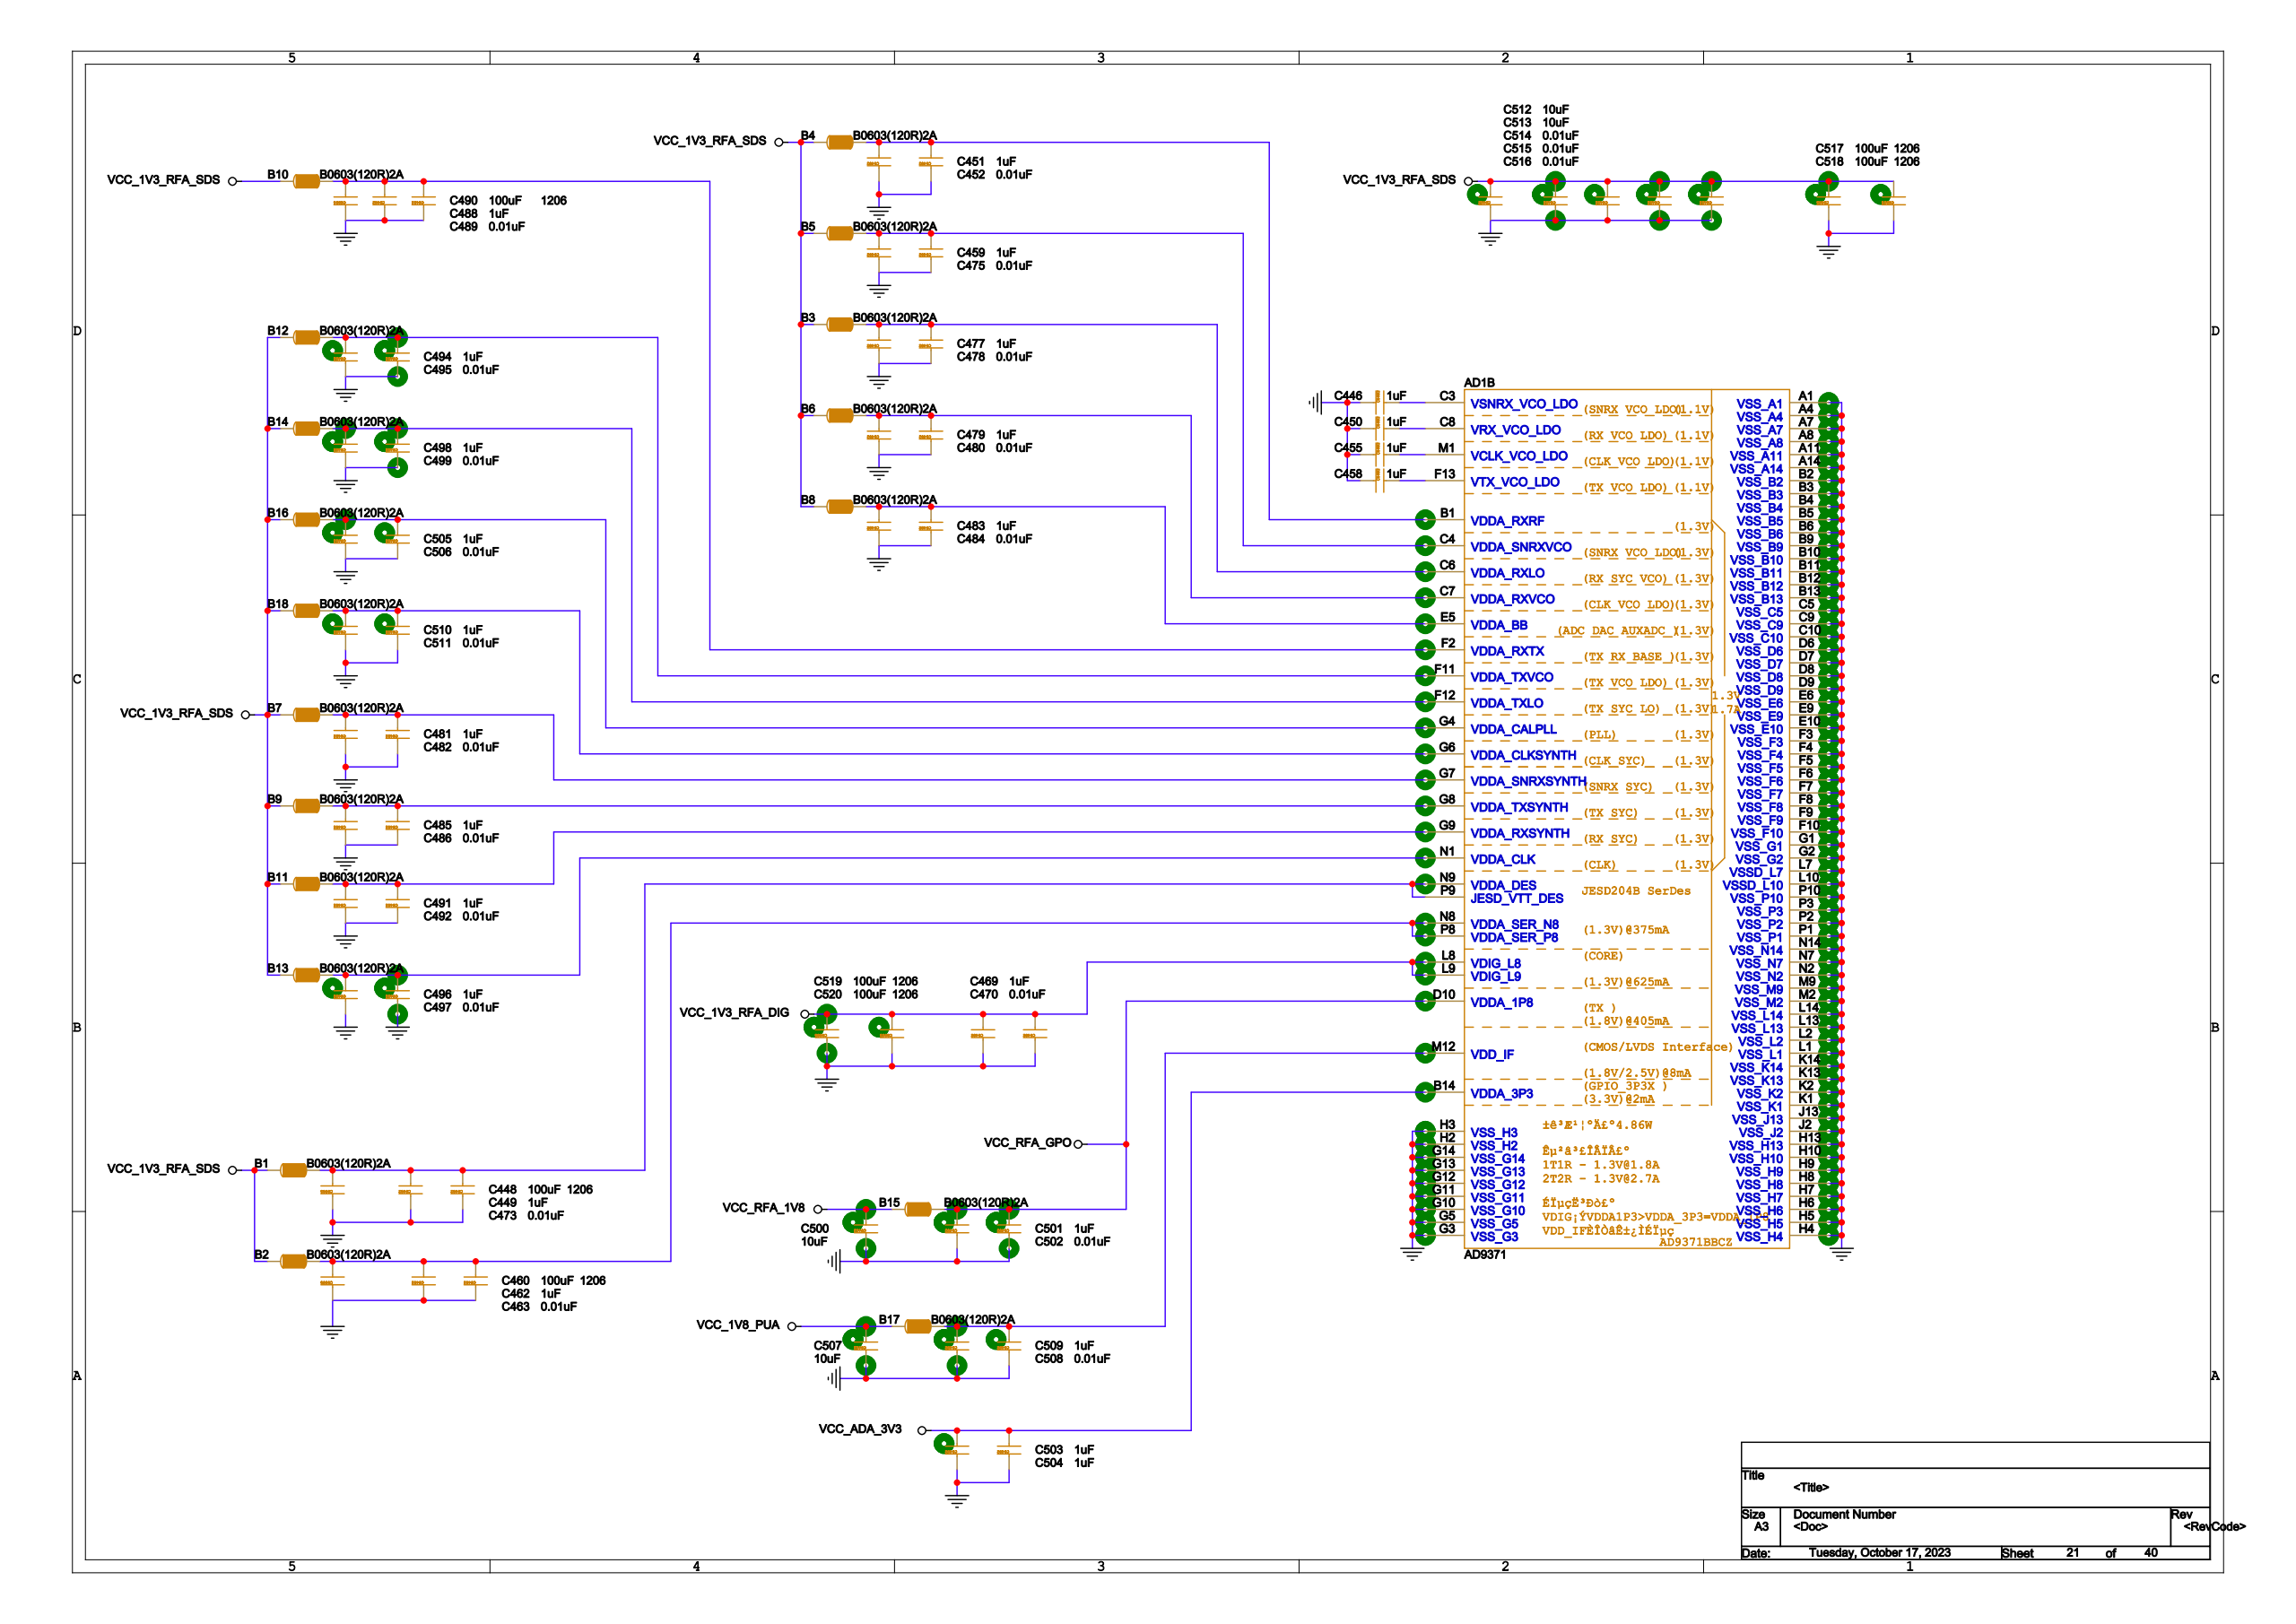Circuit board | Cadence Allegro | 1793 parts | 1223 nets | one sheet of the schematic
Parts on this sheet (reference | value | footprint):
AD1 | AD9371 | BGA196
B1 | B0603(120R)2A | B0603
B2 | B0603(120R)2A | B0603
B3 | B0603(120R)2A | B0603
B4 | B0603(120R)2A | B0603
B5 | B0603(120R)2A | B0603
B6 | B0603(120R)2A | B0603
B7 | B0603(120R)2A | B0603
B8 | B0603(120R)2A | B0603
B9 | B0603(120R)2A | B0603
B10 | B0603(120R)2A | B0603
B11 | B0603(120R)2A | B0603
B12 | B0603(120R)2A | B0603
B13 | B0603(120R)2A | B0603
B14 | B0603(120R)2A | B0603
B15 | B0603(120R)2A | B0603
B16 | B0603(120R)2A | B0603
B17 | B0603(120R)2A | B0603
B18 | B0603(120R)2A | B0603
C446 | 1uF | C0402
C448 | 100uF | 1206
C449 | 1uF | C0402
C450 | 1uF | C0402
C451 | 1uF | C0402
C452 | 0.01uF | C0402
C455 | 1uF | C0402
C458 | 1uF | C0402
C459 | 1uF | C0402
C460 | 100uF | 1206
C462 | 1uF | C0402
C463 | 0.01uF | C0402
C469 | 1uF | C0402
C470 | 0.01uF | C0402
C473 | 0.01uF | C0402
C475 | 0.01uF | C0402
C477 | 1uF | C0402
C478 | 0.01uF | C0402
C479 | 1uF | C0402
C480 | 0.01uF | C0402
C481 | 1uF | C0402
C482 | 0.01uF | C0402
C483 | 1uF | C0402
C484 | 0.01uF | C0402
C485 | 1uF | C0402
C486 | 0.01uF | C0402
C488 | 1uF | C0402
C489 | 0.01uF | C0402
C490 | 100uF | 1206
C491 | 1uF | C0402
C492 | 0.01uF | C0402
C494 | 1uF | C0402
C495 | 0.01uF | C0402
C496 | 1uF | C0402
C497 | 0.01uF | C0402
C498 | 1uF | C0402
C499 | 0.01uF | C0402
C500 | 10uF | C0402
C501 | 1uF | C0402
C502 | 0.01uF | C0402
C503 | 1uF | C0402
C504 | 1uF | C0402
C505 | 1uF | C0402
C506 | 0.01uF | C0402
C507 | 10uF | C0402
C508 | 0.01uF | C0402
C509 | 1uF | C0402
C510 | 1uF | C0402
C511 | 0.01uF | C0402
C512 | 10uF | C0402
C513 | 10uF | C0402
C514 | 0.01uF | C0402
C515 | 0.01uF | C0402
C516 | 0.01uF | C0402
C517 | 100uF | 1206
C518 | 100uF | 1206
C519 | 100uF | 1206
C520 | 100uF | 1206
Nets of these parts (net: part-pin ...):
GND: C446-1 C448-1 C449-1 C450-1 C451-1 C452-1 C455-1 C458-1 C459-1 C460-1 C462-1 C463-1 C469-1 C470-1 C473-1 C475-1 C477-1 C478-1 C479-1 C480-1 C481-1 C482-1 C483-1 C484-1 C485-1 C486-1 C488-1 C489-1 C490-1 C491-1 C492-1 C494-1 C495-1 C496-1 C497-1 C498-1 C499-1 C500-1 C501-1 C502-1 C503-1 C504-1 C505-1 C506-1 C507-1 C508-1 C509-1 C510-1 C511-1 C512-1 C513-1 C514-1 C515-1 C516-1 C517-1 C518-1 C519-1 C520-1 AD1-A1 AD1-A4 AD1-A7 AD1-A8 AD1-A11 AD1-A14 AD1-B2 AD1-B3 AD1-B4 AD1-B5 AD1-B6 AD1-B9 AD1-B10 AD1-B11 AD1-B12 AD1-B13 AD1-C5 AD1-C9 AD1-C10 AD1-D6 AD1-D7 AD1-D8 AD1-D9 AD1-E6 AD1-E9 AD1-E10 AD1-F3 AD1-F4 AD1-F5 AD1-F6 AD1-F7 AD1-F8 AD1-F9 AD1-F10 AD1-G1 AD1-G2 AD1-G3 AD1-G5 AD1-G10 AD1-G11 AD1-G12 AD1-G13 AD1-G14 AD1-H2 AD1-H3 AD1-H4 AD1-H5 AD1-H6 AD1-H7 AD1-H8 AD1-H9 AD1-H10 AD1-H13 AD1-J2 AD1-J13 AD1-K1 AD1-K2 AD1-K13 AD1-K14 AD1-L1 AD1-L2 AD1-L7 AD1-L10 AD1-L13 AD1-L14 AD1-M2 AD1-M9 AD1-N2 AD1-N7 AD1-N14 AD1-P1 AD1-P2 AD1-P3 AD1-P10
N16736626: B1-2 C448-2 C449-2 C473-2 AD1-N9 AD1-P9
N16736756: B2-2 C460-2 C462-2 C463-2 AD1-N8 AD1-P8
N16736874: B10-2 C488-2 C489-2 C490-2 AD1-F2
VCC_1V3_RFA_SDS: B1-1 B2-1 B3-1 B4-1 B5-1 B6-1 B7-1 B8-1 B9-1 B10-1 B11-1 B12-1 B13-1 B14-1 B16-1 B18-1 C512-2 C513-2 C514-2 C515-2 C516-2 C517-2 C518-2
VCC_1V3_RFA_DIG: C469-2 C470-2 C519-2 C520-2 AD1-L8 AD1-L9
VCC_RFA_1V8: B15-1 C500-2
VCC_1V8_PUA: B17-1 C507-2
VCC_ADA_3V3: C503-2 C504-2 AD1-B14
N16736716: C455-2 AD1-M1
VCC_RFA_GPO: B15-2 C501-2 C502-2 AD1-D10
N16736860: B8-2 C483-2 C484-2 AD1-E5
N16736944: B16-2 C505-2 C506-2 AD1-G4
N16737074: B13-2 C496-2 C497-2 AD1-N1
N16736970: B18-2 C510-2 C511-2 AD1-G6
N16736816: B3-2 C477-2 C478-2 AD1-C6
N16736614: B4-2 C451-2 C452-2 AD1-B1
N16737042: B11-2 C491-2 C492-2 AD1-G9
N16736840: B6-2 C479-2 C480-2 AD1-C7
N16736904: B7-2 C481-2 C482-2 AD1-G7
N16736748: B5-2 C459-2 C475-2 AD1-C4
N16736914: B14-2 C498-2 C499-2 AD1-F12
N16737000: B9-2 C485-2 C486-2 AD1-G8
N16736894: B12-2 C494-2 C495-2 AD1-F11
N16737382: B17-2 C508-2 C509-2 AD1-M12
N16736670: C450-2 AD1-C8
N16736646: C446-2 AD1-C3
N16736738: C458-2 AD1-F13